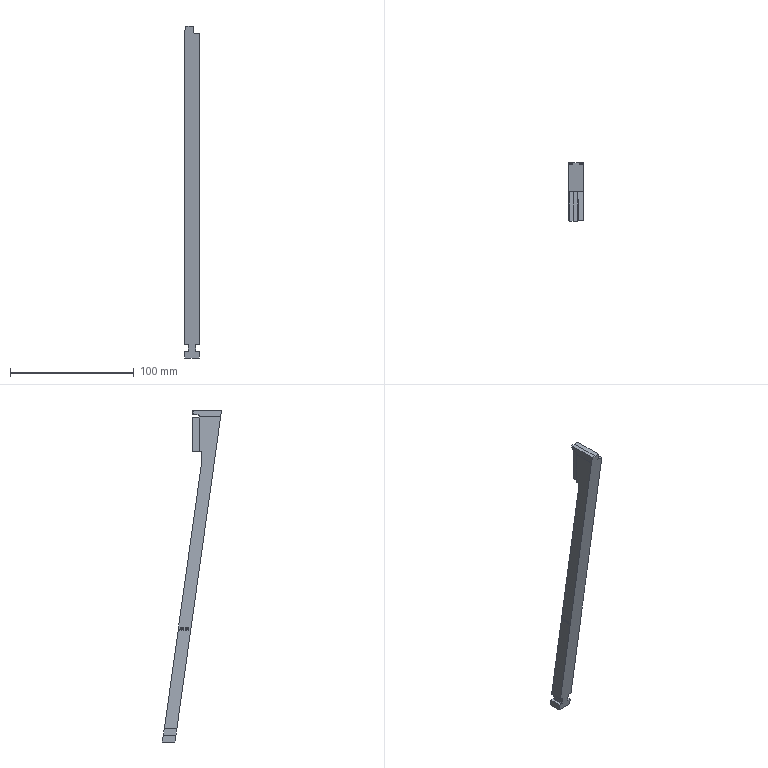Part | Creo | 1 solid | 131 faces | box 12 x 47.744 x 267.86 mm | volume 35542 mm3 | other 77 | plane 47 | cylinder 7 | commonest cylinder face diameters 1 x4 1.567 x1 2 x1 24.717 x1